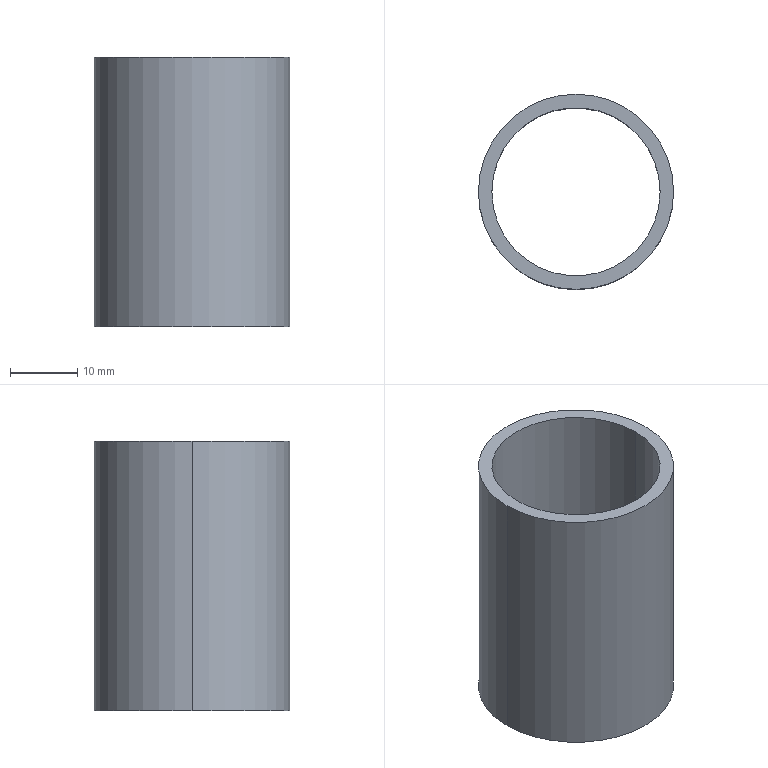Part | SolidWorks | features Extrusion 1 | 1 solid | 6 faces | box 29 x 29 x 40 mm | volume 6786 mm3 | cylinder 4 | plane 2 | commonest cylinder face diameters 25 x2 29 x2
STEP:
#1=CARTESIAN_POINT('',(-12.5,0.,40.));
#2=VERTEX_POINT('',#1);
#3=CARTESIAN_POINT('',(12.5,0.,40.));
#4=VERTEX_POINT('',#3);
#5=CARTESIAN_POINT('',(0.,0.,40.));
#6=DIRECTION('',(0.,0.,1.));
#7=DIRECTION('',(1.,0.,0.));
#8=AXIS2_PLACEMENT_3D('',#5,#6,#7);
#9=CIRCLE('',#8,12.5);
#10=EDGE_CURVE('',#2,#4,#9,.T.);
#11=ORIENTED_EDGE('',*,*,#10,.T.);
#12=CARTESIAN_POINT('',(12.5,0.,0.));
#13=VERTEX_POINT('',#12);
#14=CARTESIAN_POINT('',(12.5,0.,40.));
#15=DIRECTION('',(0.,0.,-1.));
#16=VECTOR('',#15,1000.);
#17=LINE('',#14,#16);
#18=EDGE_CURVE('',#4,#13,#17,.T.);
#19=ORIENTED_EDGE('',*,*,#18,.T.);
#20=CARTESIAN_POINT('',(-12.5,0.,0.));
#21=VERTEX_POINT('',#20);
#22=CARTESIAN_POINT('',(0.,0.,0.));
#23=DIRECTION('',(0.,0.,1.));
#24=DIRECTION('',(1.,0.,0.));
#25=AXIS2_PLACEMENT_3D('',#22,#23,#24);
#26=CIRCLE('',#25,12.5);
#27=EDGE_CURVE('',#21,#13,#26,.T.);
#28=ORIENTED_EDGE('',*,*,#27,.F.);
#29=CARTESIAN_POINT('',(-12.5,0.,40.));
#30=DIRECTION('',(0.,0.,-1.));
#31=VECTOR('',#30,1000.);
#32=LINE('',#29,#31);
#33=EDGE_CURVE('',#2,#21,#32,.T.);
#34=ORIENTED_EDGE('',*,*,#33,.F.);
#35=EDGE_LOOP('',(#11,#19,#28,#34));
#36=FACE_OUTER_BOUND('',#35,.T.);
#37=CARTESIAN_POINT('',(0.,0.,40.));
#38=DIRECTION('',(0.,0.,-1.));
#39=DIRECTION('',(-1.,0.,0.));
#40=AXIS2_PLACEMENT_3D('',#37,#38,#39);
#41=CYLINDRICAL_SURFACE('',#40,12.5);
#42=ADVANCED_FACE('',(#36),#41,.F.);
#43=CARTESIAN_POINT('',(14.5,0.,40.));
#44=VERTEX_POINT('',#43);
#45=CARTESIAN_POINT('',(-14.5,0.,40.));
#46=VERTEX_POINT('',#45);
#47=CARTESIAN_POINT('',(0.,0.,40.));
#48=DIRECTION('',(0.,0.,1.));
#49=DIRECTION('',(1.,0.,0.));
#50=AXIS2_PLACEMENT_3D('',#47,#48,#49);
#51=CIRCLE('',#50,14.5);
#52=EDGE_CURVE('',#44,#46,#51,.T.);
#53=ORIENTED_EDGE('',*,*,#52,.F.);
#54=CARTESIAN_POINT('',(14.5,0.,0.));
#55=VERTEX_POINT('',#54);
#56=CARTESIAN_POINT('',(14.5,0.,40.));
#57=DIRECTION('',(0.,0.,-1.));
#58=VECTOR('',#57,1000.);
#59=LINE('',#56,#58);
#60=EDGE_CURVE('',#44,#55,#59,.T.);
#61=ORIENTED_EDGE('',*,*,#60,.T.);
#62=CARTESIAN_POINT('',(-14.5,0.,0.));
#63=VERTEX_POINT('',#62);
#64=CARTESIAN_POINT('',(0.,0.,0.));
#65=DIRECTION('',(0.,0.,1.));
#66=DIRECTION('',(1.,0.,0.));
#67=AXIS2_PLACEMENT_3D('',#64,#65,#66);
#68=CIRCLE('',#67,14.5);
#69=EDGE_CURVE('',#55,#63,#68,.T.);
#70=ORIENTED_EDGE('',*,*,#69,.T.);
#71=CARTESIAN_POINT('',(-14.5,0.,40.));
#72=DIRECTION('',(0.,0.,-1.));
#73=VECTOR('',#72,1000.);
#74=LINE('',#71,#73);
#75=EDGE_CURVE('',#46,#63,#74,.T.);
#76=ORIENTED_EDGE('',*,*,#75,.F.);
#77=EDGE_LOOP('',(#53,#61,#70,#76));
#78=FACE_OUTER_BOUND('',#77,.T.);
#79=CARTESIAN_POINT('',(0.,0.,40.));
#80=DIRECTION('',(0.,0.,-1.));
#81=DIRECTION('',(-1.,0.,0.));
#82=AXIS2_PLACEMENT_3D('',#79,#80,#81);
#83=CYLINDRICAL_SURFACE('',#82,14.5);
#84=ADVANCED_FACE('',(#78),#83,.T.);
#85=CARTESIAN_POINT('',(0.,0.,40.));
#86=DIRECTION('',(0.,0.,1.));
#87=DIRECTION('',(1.,0.,0.));
#88=AXIS2_PLACEMENT_3D('',#85,#86,#87);
#89=CIRCLE('',#88,14.5);
#90=EDGE_CURVE('',#46,#44,#89,.T.);
#91=ORIENTED_EDGE('',*,*,#90,.T.);
#92=ORIENTED_EDGE('',*,*,#52,.T.);
#93=EDGE_LOOP('',(#91,#92));
#94=FACE_OUTER_BOUND('',#93,.T.);
#95=ORIENTED_EDGE('',*,*,#10,.F.);
#96=CARTESIAN_POINT('',(0.,0.,40.));
#97=DIRECTION('',(0.,0.,1.));
#98=DIRECTION('',(1.,0.,0.));
#99=AXIS2_PLACEMENT_3D('',#96,#97,#98);
#100=CIRCLE('',#99,12.5);
#101=EDGE_CURVE('',#4,#2,#100,.T.);
#102=ORIENTED_EDGE('',*,*,#101,.F.);
#103=EDGE_LOOP('',(#95,#102));
#104=FACE_BOUND('',#103,.T.);
#105=CARTESIAN_POINT('',(0.,0.,40.));
#106=DIRECTION('',(0.,0.,1.));
#107=DIRECTION('',(1.,0.,0.));
#108=AXIS2_PLACEMENT_3D('',#105,#106,#107);
#109=PLANE('',#108);
#110=ADVANCED_FACE('',(#94,#104),#109,.T.);
#111=CARTESIAN_POINT('',(0.,0.,0.));
#112=DIRECTION('',(0.,0.,1.));
#113=DIRECTION('',(1.,0.,0.));
#114=AXIS2_PLACEMENT_3D('',#111,#112,#113);
#115=CIRCLE('',#114,14.5);
#116=EDGE_CURVE('',#63,#55,#115,.T.);
#117=ORIENTED_EDGE('',*,*,#116,.F.);
#118=ORIENTED_EDGE('',*,*,#69,.F.);
#119=EDGE_LOOP('',(#117,#118));
#120=FACE_OUTER_BOUND('',#119,.T.);
#121=ORIENTED_EDGE('',*,*,#27,.T.);
#122=CARTESIAN_POINT('',(0.,0.,0.));
#123=DIRECTION('',(0.,0.,1.));
#124=DIRECTION('',(1.,0.,0.));
#125=AXIS2_PLACEMENT_3D('',#122,#123,#124);
#126=CIRCLE('',#125,12.5);
#127=EDGE_CURVE('',#13,#21,#126,.T.);
#128=ORIENTED_EDGE('',*,*,#127,.T.);
#129=EDGE_LOOP('',(#121,#128));
#130=FACE_BOUND('',#129,.T.);
#131=CARTESIAN_POINT('',(0.,0.,0.));
#132=DIRECTION('',(0.,0.,1.));
#133=DIRECTION('',(1.,0.,0.));
#134=AXIS2_PLACEMENT_3D('',#131,#132,#133);
#135=PLANE('',#134);
#136=ADVANCED_FACE('',(#120,#130),#135,.F.);
#137=ORIENTED_EDGE('',*,*,#60,.F.);
#138=ORIENTED_EDGE('',*,*,#90,.F.);
#139=ORIENTED_EDGE('',*,*,#75,.T.);
#140=ORIENTED_EDGE('',*,*,#116,.T.);
#141=EDGE_LOOP('',(#137,#138,#139,#140));
#142=FACE_OUTER_BOUND('',#141,.T.);
#143=CARTESIAN_POINT('',(0.,0.,40.));
#144=DIRECTION('',(0.,0.,-1.));
#145=DIRECTION('',(-1.,0.,0.));
#146=AXIS2_PLACEMENT_3D('',#143,#144,#145);
#147=CYLINDRICAL_SURFACE('',#146,14.5);
#148=ADVANCED_FACE('',(#142),#147,.T.);
#149=ORIENTED_EDGE('',*,*,#18,.F.);
#150=ORIENTED_EDGE('',*,*,#101,.T.);
#151=ORIENTED_EDGE('',*,*,#33,.T.);
#152=ORIENTED_EDGE('',*,*,#127,.F.);
#153=EDGE_LOOP('',(#149,#150,#151,#152));
#154=FACE_OUTER_BOUND('',#153,.T.);
#155=CARTESIAN_POINT('',(0.,0.,40.));
#156=DIRECTION('',(0.,0.,-1.));
#157=DIRECTION('',(-1.,0.,0.));
#158=AXIS2_PLACEMENT_3D('',#155,#156,#157);
#159=CYLINDRICAL_SURFACE('',#158,12.5);
#160=ADVANCED_FACE('',(#154),#159,.F.);
#161=CLOSED_SHELL('',(#42,#84,#110,#136,#148,#160));
#162=MANIFOLD_SOLID_BREP('',#161);
#163=CARTESIAN_POINT('',(0.,0.,0.));
#164=DIRECTION('',(0.,0.,1.));
#165=DIRECTION('',(1.,0.,0.));
#166=AXIS2_PLACEMENT_3D('',#163,#164,#165);
#167=(LENGTH_UNIT()NAMED_UNIT(*)SI_UNIT(.MILLI.,.METRE.));
#168=UNCERTAINTY_MEASURE_WITH_UNIT(LENGTH_MEASURE(0.00001),#167,'','');
#169=(NAMED_UNIT(*)PLANE_ANGLE_UNIT()SI_UNIT($,.RADIAN.));
#170=(NAMED_UNIT(*)SI_UNIT($,.STERADIAN.)SOLID_ANGLE_UNIT());
#171=(GEOMETRIC_REPRESENTATION_CONTEXT(3)GLOBAL_UNCERTAINTY_ASSIGNED_CONTEXT((#168))GLOBAL_UNIT_ASSIGNED_CONTEXT((#167,#169,#170))REPRESENTATION_CONTEXT('',''));
#172=ADVANCED_BREP_SHAPE_REPRESENTATION('',(#162,#166),#171);